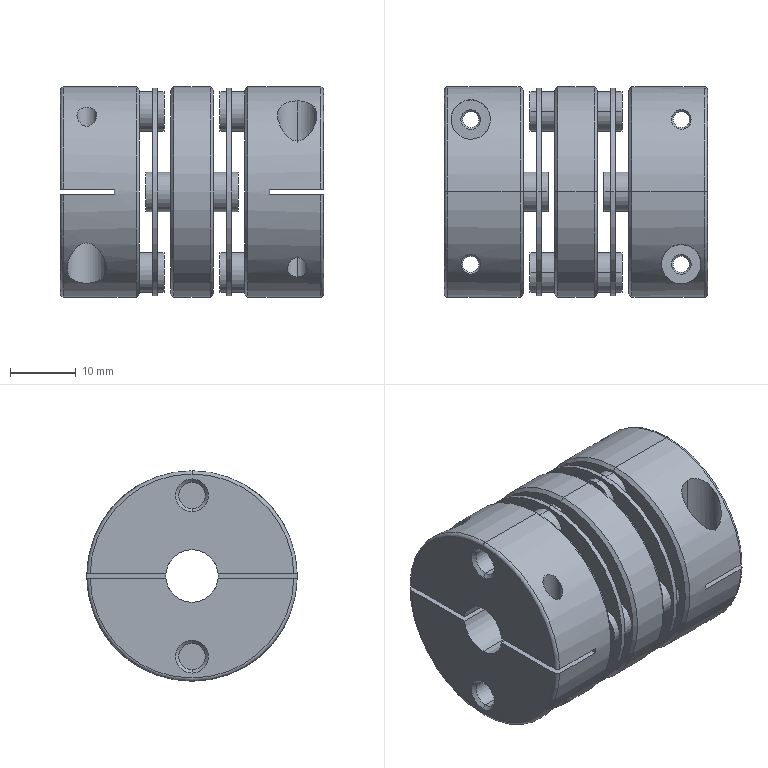Part | NX | features BREP 1 | 1 solid | 170 faces | box 40 x 32 x 32 mm | volume 21113 mm3 | cylinder 92 | plane 40 | cone 32 | torus 6 | commonest cylinder face diameters 6 x40 3 x16 2.459 x8 4 x8 16 x6 32 x6